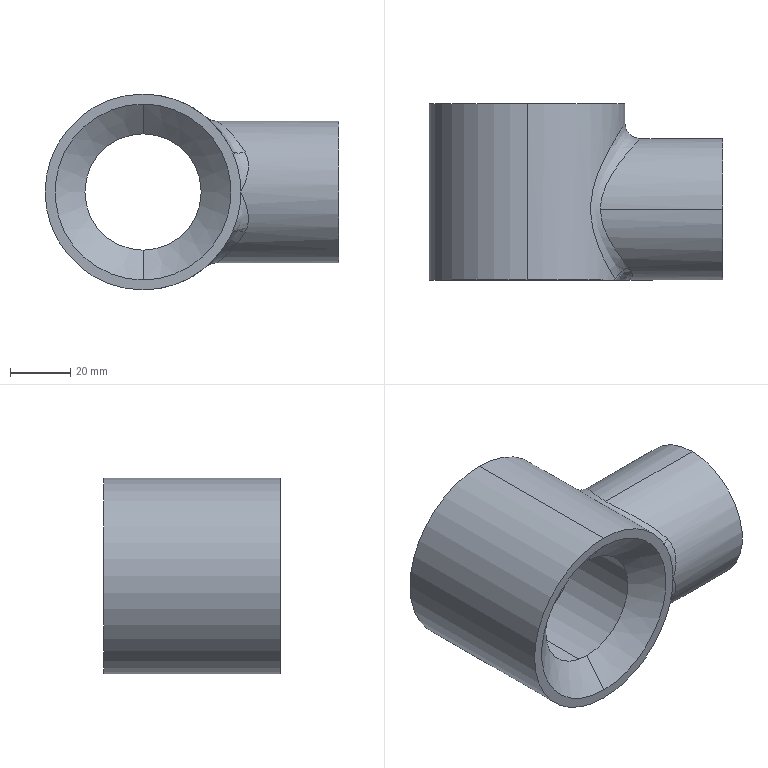Part | SolidWorks | features RevCut 2, Fillet 1, ICE 1, RefAxis 1, Revolution 1 | 1 solid | 24 faces | box 97.5 x 58.5 x 65 mm | volume 121615 mm3 | cylinder 12 | plane 7 | spline 3 | cone 2 | commonest cylinder face diameters 34 x2 39 x2 45 x2 47 x2 48 x2 65 x2